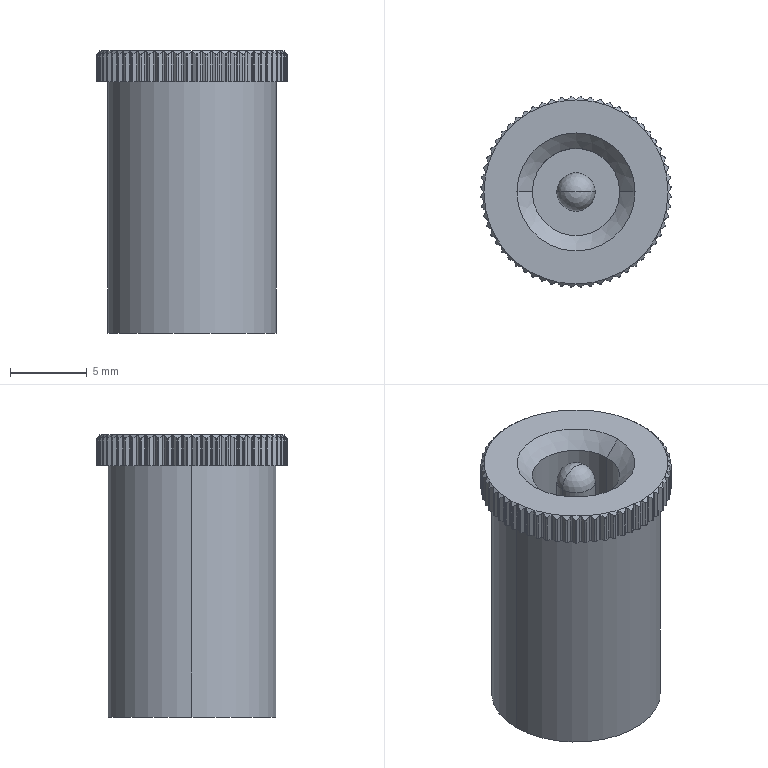Part | NX | features BREP 1 | 1 solid | 283 faces | box 12.424 x 12.424 x 18.4 mm | volume 1636 mm3 | cylinder 153 | plane 124 | cone 4 | sphere 2 | commonest cylinder face diameters 0.2 x147 2.5 x2 5.7 x2 11 x2